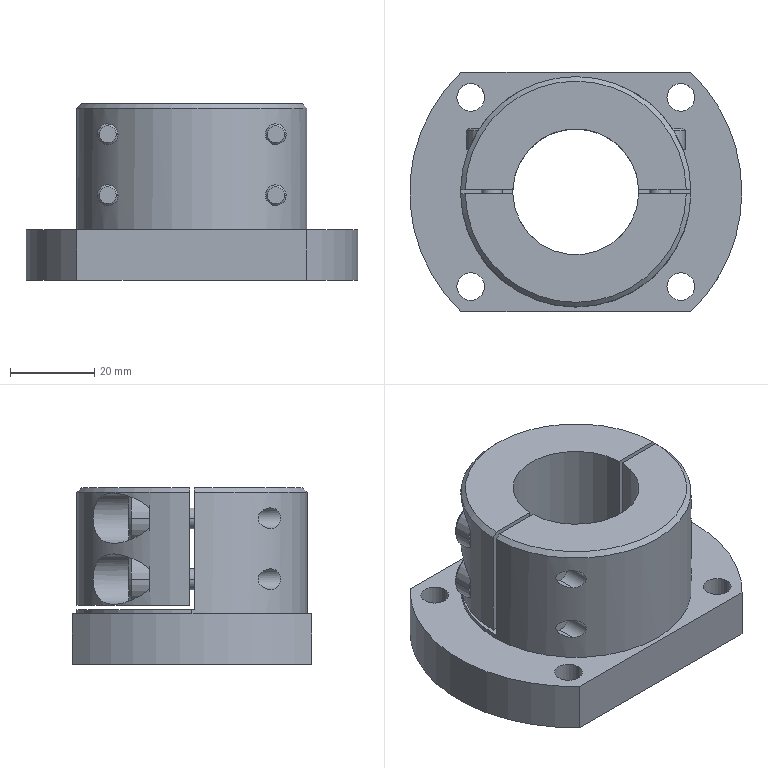Part | STEP file | 001-004-GAY12_D30 | 6 solids | 135 faces | box 79 x 57 x 42 mm | volume 84373 mm3 | cylinder 61 | plane 56 | cone 18 | commonest cylinder face diameters 12 x20 6.6 x16 4.917 x8 5 x8 30 x3 54.8 x3